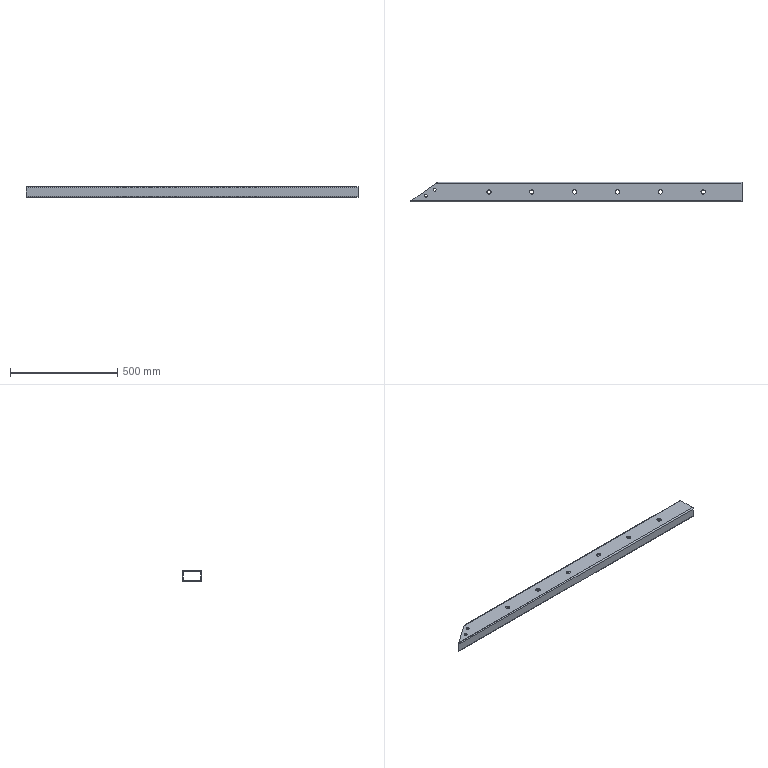Part | SolidWorks | features HoleWzd 2, LPattern 1, Split 1, WeldMemberFeat 1, WeldmentFeature 1 | 1 solid | 50 faces | box 1550 x 90 x 50 mm | volume 1146938 mm3 | cylinder 40 | plane 10 | commonest cylinder face diameters 20 x24 14 x8 6 x4 12 x4